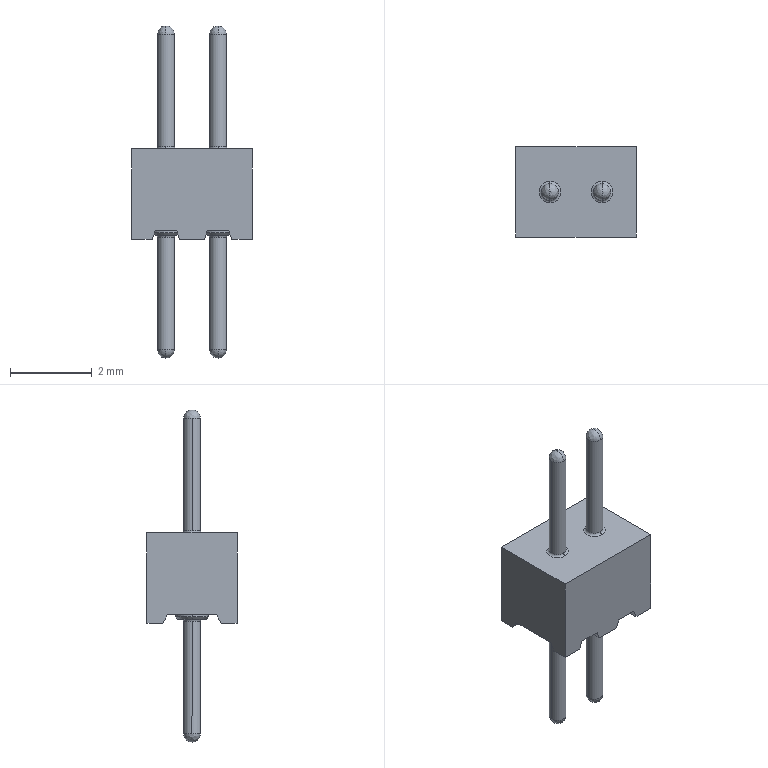Part | STEP file | RJ-USIO-V1_2-220411_4 | 1 solid | 64 faces | box 2.95 x 2.2 x 8.1 mm | volume 14.941 mm3 | plane 28 | spline 12 | cylinder 12 | torus 8 | cone 4 | commonest cylinder face diameters 0.41 x8 0.805 x4